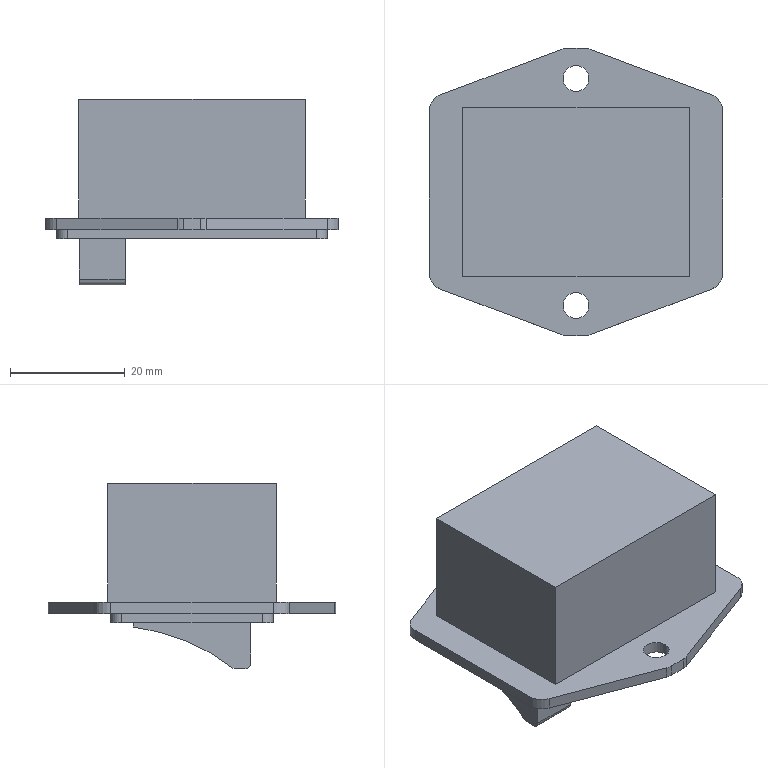Part | SolidWorks | features MirrorStock 1 | 1 solid | 50 faces | box 51 x 50 x 32.3 mm | volume 28039 mm3 | plane 32 | cylinder 18 | commonest cylinder face diameters 6 x8 4 x4 4.5 x4 2 x1 73.633 x1
STEP:
#1=CARTESIAN_POINT('',(2.25,-19.75,-20.7));
#2=VERTEX_POINT('',#1);
#3=CARTESIAN_POINT('',(-2.25,-19.75,-20.7));
#4=VERTEX_POINT('',#3);
#5=CARTESIAN_POINT('',(0.,-19.75,-20.7));
#6=DIRECTION('',(0.,0.,1.));
#7=DIRECTION('',(1.,0.,0.));
#8=AXIS2_PLACEMENT_3D('',#5,#6,#7);
#9=CIRCLE('',#8,2.25);
#10=EDGE_CURVE('',#2,#4,#9,.T.);
#11=ORIENTED_EDGE('',*,*,#10,.T.);
#12=CARTESIAN_POINT('',(-2.25,-19.75,-22.7));
#13=VERTEX_POINT('',#12);
#14=CARTESIAN_POINT('',(-2.25,-19.75,0.));
#15=DIRECTION('',(0.,0.,-1.));
#16=VECTOR('',#15,1000.);
#17=LINE('',#14,#16);
#18=EDGE_CURVE('',#4,#13,#17,.T.);
#19=ORIENTED_EDGE('',*,*,#18,.T.);
#20=CARTESIAN_POINT('',(2.25,-19.75,-22.7));
#21=VERTEX_POINT('',#20);
#22=CARTESIAN_POINT('',(0.,-19.75,-22.7));
#23=DIRECTION('',(0.,0.,1.));
#24=DIRECTION('',(1.,0.,0.));
#25=AXIS2_PLACEMENT_3D('',#22,#23,#24);
#26=CIRCLE('',#25,2.25);
#27=EDGE_CURVE('',#21,#13,#26,.T.);
#28=ORIENTED_EDGE('',*,*,#27,.F.);
#29=CARTESIAN_POINT('',(2.25,-19.75,0.));
#30=DIRECTION('',(0.,0.,-1.));
#31=VECTOR('',#30,1000.);
#32=LINE('',#29,#31);
#33=EDGE_CURVE('',#2,#21,#32,.T.);
#34=ORIENTED_EDGE('',*,*,#33,.F.);
#35=EDGE_LOOP('',(#11,#19,#28,#34));
#36=FACE_OUTER_BOUND('',#35,.T.);
#37=CARTESIAN_POINT('',(0.,-19.75,0.));
#38=DIRECTION('',(0.,0.,-1.));
#39=DIRECTION('',(1.,0.,0.));
#40=AXIS2_PLACEMENT_3D('',#37,#38,#39);
#41=CYLINDRICAL_SURFACE('',#40,2.25);
#42=ADVANCED_FACE('',(#36),#41,.F.);
#43=CARTESIAN_POINT('',(2.25,19.75,-20.7));
#44=VERTEX_POINT('',#43);
#45=CARTESIAN_POINT('',(-2.25,19.75,-20.7));
#46=VERTEX_POINT('',#45);
#47=CARTESIAN_POINT('',(0.,19.75,-20.7));
#48=DIRECTION('',(0.,0.,1.));
#49=DIRECTION('',(1.,0.,0.));
#50=AXIS2_PLACEMENT_3D('',#47,#48,#49);
#51=CIRCLE('',#50,2.25);
#52=EDGE_CURVE('',#44,#46,#51,.T.);
#53=ORIENTED_EDGE('',*,*,#52,.T.);
#54=CARTESIAN_POINT('',(-2.25,19.75,-22.7));
#55=VERTEX_POINT('',#54);
#56=CARTESIAN_POINT('',(-2.25,19.75,0.));
#57=DIRECTION('',(0.,0.,-1.));
#58=VECTOR('',#57,1000.);
#59=LINE('',#56,#58);
#60=EDGE_CURVE('',#46,#55,#59,.T.);
#61=ORIENTED_EDGE('',*,*,#60,.T.);
#62=CARTESIAN_POINT('',(2.25,19.75,-22.7));
#63=VERTEX_POINT('',#62);
#64=CARTESIAN_POINT('',(0.,19.75,-22.7));
#65=DIRECTION('',(0.,0.,1.));
#66=DIRECTION('',(1.,0.,0.));
#67=AXIS2_PLACEMENT_3D('',#64,#65,#66);
#68=CIRCLE('',#67,2.25);
#69=EDGE_CURVE('',#63,#55,#68,.T.);
#70=ORIENTED_EDGE('',*,*,#69,.F.);
#71=CARTESIAN_POINT('',(2.25,19.75,0.));
#72=DIRECTION('',(0.,0.,-1.));
#73=VECTOR('',#72,1000.);
#74=LINE('',#71,#73);
#75=EDGE_CURVE('',#44,#63,#74,.T.);
#76=ORIENTED_EDGE('',*,*,#75,.F.);
#77=EDGE_LOOP('',(#53,#61,#70,#76));
#78=FACE_OUTER_BOUND('',#77,.T.);
#79=CARTESIAN_POINT('',(0.,19.75,0.));
#80=DIRECTION('',(0.,0.,-1.));
#81=DIRECTION('',(1.,0.,0.));
#82=AXIS2_PLACEMENT_3D('',#79,#80,#81);
#83=CYLINDRICAL_SURFACE('',#82,2.25);
#84=ADVANCED_FACE('',(#78),#83,.F.);
#85=CARTESIAN_POINT('',(-21.6,-14.2,-24.3));
#86=VERTEX_POINT('',#85);
#87=CARTESIAN_POINT('',(21.6,-14.2,-24.3));
#88=VERTEX_POINT('',#87);
#89=CARTESIAN_POINT('',(23.6,-14.2,-24.3));
#90=DIRECTION('',(1.,0.,0.));
#91=VECTOR('',#90,1000.);
#92=LINE('',#89,#91);
#93=EDGE_CURVE('',#86,#88,#92,.T.);
#94=ORIENTED_EDGE('',*,*,#93,.F.);
#95=CARTESIAN_POINT('',(-23.6,-12.2,-24.3));
#96=VERTEX_POINT('',#95);
#97=CARTESIAN_POINT('',(-21.6,-12.2,-24.3));
#98=DIRECTION('',(0.,0.,1.));
#99=DIRECTION('',(1.,0.,0.));
#100=AXIS2_PLACEMENT_3D('',#97,#98,#99);
#101=CIRCLE('',#100,2.);
#102=EDGE_CURVE('',#96,#86,#101,.T.);
#103=ORIENTED_EDGE('',*,*,#102,.F.);
#104=CARTESIAN_POINT('',(-23.6,12.2,-24.3));
#105=VERTEX_POINT('',#104);
#106=CARTESIAN_POINT('',(-23.6,-14.2,-24.3));
#107=DIRECTION('',(0.,-1.,0.));
#108=VECTOR('',#107,1000.);
#109=LINE('',#106,#108);
#110=EDGE_CURVE('',#105,#96,#109,.T.);
#111=ORIENTED_EDGE('',*,*,#110,.F.);
#112=CARTESIAN_POINT('',(-21.6,14.2,-24.3));
#113=VERTEX_POINT('',#112);
#114=CARTESIAN_POINT('',(-21.6,12.2,-24.3));
#115=DIRECTION('',(0.,0.,1.));
#116=DIRECTION('',(1.,0.,0.));
#117=AXIS2_PLACEMENT_3D('',#114,#115,#116);
#118=CIRCLE('',#117,2.);
#119=EDGE_CURVE('',#113,#105,#118,.T.);
#120=ORIENTED_EDGE('',*,*,#119,.F.);
#121=CARTESIAN_POINT('',(21.6,14.2,-24.3));
#122=VERTEX_POINT('',#121);
#123=CARTESIAN_POINT('',(23.6,14.2,-24.3));
#124=DIRECTION('',(-1.,0.,0.));
#125=VECTOR('',#124,1000.);
#126=LINE('',#123,#125);
#127=EDGE_CURVE('',#122,#113,#126,.T.);
#128=ORIENTED_EDGE('',*,*,#127,.F.);
#129=CARTESIAN_POINT('',(23.6,12.2,-24.3));
#130=VERTEX_POINT('',#129);
#131=CARTESIAN_POINT('',(21.6,12.2,-24.3));
#132=DIRECTION('',(0.,0.,1.));
#133=DIRECTION('',(1.,0.,0.));
#134=AXIS2_PLACEMENT_3D('',#131,#132,#133);
#135=CIRCLE('',#134,2.);
#136=EDGE_CURVE('',#130,#122,#135,.T.);
#137=ORIENTED_EDGE('',*,*,#136,.F.);
#138=CARTESIAN_POINT('',(23.6,-12.2,-24.3));
#139=VERTEX_POINT('',#138);
#140=CARTESIAN_POINT('',(23.6,-14.2,-24.3));
#141=DIRECTION('',(0.,1.,0.));
#142=VECTOR('',#141,1000.);
#143=LINE('',#140,#142);
#144=EDGE_CURVE('',#139,#130,#143,.T.);
#145=ORIENTED_EDGE('',*,*,#144,.F.);
#146=CARTESIAN_POINT('',(21.6,-12.2,-24.3));
#147=DIRECTION('',(0.,0.,1.));
#148=DIRECTION('',(1.,0.,0.));
#149=AXIS2_PLACEMENT_3D('',#146,#147,#148);
#150=CIRCLE('',#149,2.);
#151=EDGE_CURVE('',#88,#139,#150,.T.);
#152=ORIENTED_EDGE('',*,*,#151,.F.);
#153=EDGE_LOOP('',(#94,#103,#111,#120,#128,#137,#145,#152));
#154=FACE_OUTER_BOUND('',#153,.T.);
#155=CARTESIAN_POINT('',(2.9,12.2,-24.3));
#156=VERTEX_POINT('',#155);
#157=CARTESIAN_POINT('',(2.9,-12.2,-24.3));
#158=VERTEX_POINT('',#157);
#159=CARTESIAN_POINT('',(2.9,0.,-24.3));
#160=DIRECTION('',(0.,-1.,0.));
#161=VECTOR('',#160,1000.);
#162=LINE('',#159,#161);
#163=EDGE_CURVE('',#156,#158,#162,.T.);
#164=ORIENTED_EDGE('',*,*,#163,.T.);
#165=CARTESIAN_POINT('',(15.9,-12.2,-24.3));
#166=VERTEX_POINT('',#165);
#167=CARTESIAN_POINT('',(0.,-12.2,-24.3));
#168=DIRECTION('',(1.,0.,0.));
#169=VECTOR('',#168,1000.);
#170=LINE('',#167,#169);
#171=EDGE_CURVE('',#158,#166,#170,.T.);
#172=ORIENTED_EDGE('',*,*,#171,.T.);
#173=CARTESIAN_POINT('',(18.9,-7.5,-24.3));
#174=VERTEX_POINT('',#173);
#175=CARTESIAN_POINT('',(16.83,-10.743,-24.3));
#176=DIRECTION('',(0.538,0.8429,0.));
#177=VECTOR('',#176,1000.);
#178=LINE('',#175,#177);
#179=EDGE_CURVE('',#166,#174,#178,.T.);
#180=ORIENTED_EDGE('',*,*,#179,.T.);
#181=CARTESIAN_POINT('',(18.9,7.5,-24.3));
#182=VERTEX_POINT('',#181);
#183=CARTESIAN_POINT('',(18.9,0.,-24.3));
#184=DIRECTION('',(0.,1.,0.));
#185=VECTOR('',#184,1000.);
#186=LINE('',#183,#185);
#187=EDGE_CURVE('',#174,#182,#186,.T.);
#188=ORIENTED_EDGE('',*,*,#187,.T.);
#189=CARTESIAN_POINT('',(15.9,12.2,-24.3));
#190=VERTEX_POINT('',#189);
#191=CARTESIAN_POINT('',(16.83,10.743,-24.3));
#192=DIRECTION('',(-0.538,0.8429,0.));
#193=VECTOR('',#192,1000.);
#194=LINE('',#191,#193);
#195=EDGE_CURVE('',#182,#190,#194,.T.);
#196=ORIENTED_EDGE('',*,*,#195,.T.);
#197=CARTESIAN_POINT('',(0.,12.2,-24.3));
#198=DIRECTION('',(1.,0.,0.));
#199=VECTOR('',#198,1000.);
#200=LINE('',#197,#199);
#201=EDGE_CURVE('',#156,#190,#200,.T.);
#202=ORIENTED_EDGE('',*,*,#201,.F.);
#203=EDGE_LOOP('',(#164,#172,#180,#188,#196,#202));
#204=FACE_BOUND('',#203,.T.);
#205=CARTESIAN_POINT('',(-19.6,-10.2,-24.3));
#206=VERTEX_POINT('',#205);
#207=CARTESIAN_POINT('',(-11.6,-10.2,-24.3));
#208=VERTEX_POINT('',#207);
#209=CARTESIAN_POINT('',(-19.6,-10.2,-24.3));
#210=DIRECTION('',(1.,0.,0.));
#211=VECTOR('',#210,1000.);
#212=LINE('',#209,#211);
#213=EDGE_CURVE('',#206,#208,#212,.T.);
#214=ORIENTED_EDGE('',*,*,#213,.T.);
#215=CARTESIAN_POINT('',(-11.6,10.2,-24.3));
#216=VERTEX_POINT('',#215);
#217=CARTESIAN_POINT('',(-11.6,10.2,-24.3));
#218=DIRECTION('',(0.,1.,0.));
#219=VECTOR('',#218,1000.);
#220=LINE('',#217,#219);
#221=EDGE_CURVE('',#208,#216,#220,.T.);
#222=ORIENTED_EDGE('',*,*,#221,.T.);
#223=CARTESIAN_POINT('',(-19.6,10.2,-24.3));
#224=VERTEX_POINT('',#223);
#225=CARTESIAN_POINT('',(-19.6,10.2,-24.3));
#226=DIRECTION('',(-1.,0.,0.));
#227=VECTOR('',#226,1000.);
#228=LINE('',#225,#227);
#229=EDGE_CURVE('',#216,#224,#228,.T.);
#230=ORIENTED_EDGE('',*,*,#229,.T.);
#231=CARTESIAN_POINT('',(-19.6,10.2,-24.3));
#232=DIRECTION('',(0.,-1.,0.));
#233=VECTOR('',#232,1000.);
#234=LINE('',#231,#233);
#235=EDGE_CURVE('',#224,#206,#234,.T.);
#236=ORIENTED_EDGE('',*,*,#235,.T.);
#237=EDGE_LOOP('',(#214,#222,#230,#236));
#238=FACE_BOUND('',#237,.T.);
#239=CARTESIAN_POINT('',(0.,0.,-24.3));
#240=DIRECTION('',(0.,0.,-1.));
#241=DIRECTION('',(1.,0.,0.));
#242=AXIS2_PLACEMENT_3D('',#239,#240,#241);
#243=PLANE('',#242);
#244=ADVANCED_FACE('',(#154,#204,#238),#243,.T.);
#245=CARTESIAN_POINT('',(-23.552,-16.929,-22.7));
#246=VERTEX_POINT('',#245);
#247=CARTESIAN_POINT('',(-2.509,-24.809,-22.7));
#248=VERTEX_POINT('',#247);
#249=CARTESIAN_POINT('',(-8.456,-22.582,-22.7));
#250=DIRECTION('',(0.9365,-0.3507,0.));
#251=VECTOR('',#250,1000.);
#252=LINE('',#249,#251);
#253=EDGE_CURVE('',#246,#248,#252,.T.);
#254=ORIENTED_EDGE('',*,*,#253,.F.);
#255=CARTESIAN_POINT('',(-25.5,-14.12,-22.7));
#256=VERTEX_POINT('',#255);
#257=CARTESIAN_POINT('',(-22.5,-14.12,-22.7));
#258=DIRECTION('',(0.,0.,1.));
#259=DIRECTION('',(1.,0.,0.));
#260=AXIS2_PLACEMENT_3D('',#257,#258,#259);
#261=CIRCLE('',#260,3.);
#262=EDGE_CURVE('',#256,#246,#261,.T.);
#263=ORIENTED_EDGE('',*,*,#262,.F.);
#264=CARTESIAN_POINT('',(-25.5,14.12,-22.7));
#265=VERTEX_POINT('',#264);
#266=CARTESIAN_POINT('',(-25.5,-25.,-22.7));
#267=DIRECTION('',(0.,-1.,0.));
#268=VECTOR('',#267,1000.);
#269=LINE('',#266,#268);
#270=EDGE_CURVE('',#265,#256,#269,.T.);
#271=ORIENTED_EDGE('',*,*,#270,.F.);
#272=CARTESIAN_POINT('',(-23.552,16.929,-22.7));
#273=VERTEX_POINT('',#272);
#274=CARTESIAN_POINT('',(-22.5,14.12,-22.7));
#275=DIRECTION('',(0.,0.,1.));
#276=DIRECTION('',(1.,0.,0.));
#277=AXIS2_PLACEMENT_3D('',#274,#275,#276);
#278=CIRCLE('',#277,3.);
#279=EDGE_CURVE('',#273,#265,#278,.T.);
#280=ORIENTED_EDGE('',*,*,#279,.F.);
#281=CARTESIAN_POINT('',(-2.509,24.809,-22.7));
#282=VERTEX_POINT('',#281);
#283=CARTESIAN_POINT('',(-8.456,22.582,-22.7));
#284=DIRECTION('',(0.9365,0.3507,0.));
#285=VECTOR('',#284,1000.);
#286=LINE('',#283,#285);
#287=EDGE_CURVE('',#273,#282,#286,.T.);
#288=ORIENTED_EDGE('',*,*,#287,.T.);
#289=CARTESIAN_POINT('',(-1.457,25.,-22.7));
#290=VERTEX_POINT('',#289);
#291=CARTESIAN_POINT('',(-1.457,22.,-22.7));
#292=DIRECTION('',(0.,0.,1.));
#293=DIRECTION('',(1.,0.,0.));
#294=AXIS2_PLACEMENT_3D('',#291,#292,#293);
#295=CIRCLE('',#294,3.);
#296=EDGE_CURVE('',#290,#282,#295,.T.);
#297=ORIENTED_EDGE('',*,*,#296,.F.);
#298=CARTESIAN_POINT('',(1.457,25.,-22.7));
#299=VERTEX_POINT('',#298);
#300=CARTESIAN_POINT('',(25.5,25.,-22.7));
#301=DIRECTION('',(-1.,0.,0.));
#302=VECTOR('',#301,1000.);
#303=LINE('',#300,#302);
#304=EDGE_CURVE('',#299,#290,#303,.T.);
#305=ORIENTED_EDGE('',*,*,#304,.F.);
#306=CARTESIAN_POINT('',(2.509,24.809,-22.7));
#307=VERTEX_POINT('',#306);
#308=CARTESIAN_POINT('',(1.457,22.,-22.7));
#309=DIRECTION('',(0.,0.,1.));
#310=DIRECTION('',(1.,0.,0.));
#311=AXIS2_PLACEMENT_3D('',#308,#309,#310);
#312=CIRCLE('',#311,3.);
#313=EDGE_CURVE('',#307,#299,#312,.T.);
#314=ORIENTED_EDGE('',*,*,#313,.F.);
#315=CARTESIAN_POINT('',(23.552,16.929,-22.7));
#316=VERTEX_POINT('',#315);
#317=CARTESIAN_POINT('',(8.456,22.582,-22.7));
#318=DIRECTION('',(-0.9365,0.3507,0.));
#319=VECTOR('',#318,1000.);
#320=LINE('',#317,#319);
#321=EDGE_CURVE('',#316,#307,#320,.T.);
#322=ORIENTED_EDGE('',*,*,#321,.F.);
#323=CARTESIAN_POINT('',(25.5,14.12,-22.7));
#324=VERTEX_POINT('',#323);
#325=CARTESIAN_POINT('',(22.5,14.12,-22.7));
#326=DIRECTION('',(0.,0.,1.));
#327=DIRECTION('',(1.,0.,0.));
#328=AXIS2_PLACEMENT_3D('',#325,#326,#327);
#329=CIRCLE('',#328,3.);
#330=EDGE_CURVE('',#324,#316,#329,.T.);
#331=ORIENTED_EDGE('',*,*,#330,.F.);
#332=CARTESIAN_POINT('',(25.5,-14.12,-22.7));
#333=VERTEX_POINT('',#332);
#334=CARTESIAN_POINT('',(25.5,-25.,-22.7));
#335=DIRECTION('',(0.,1.,0.));
#336=VECTOR('',#335,1000.);
#337=LINE('',#334,#336);
#338=EDGE_CURVE('',#333,#324,#337,.T.);
#339=ORIENTED_EDGE('',*,*,#338,.F.);
#340=CARTESIAN_POINT('',(23.552,-16.929,-22.7));
#341=VERTEX_POINT('',#340);
#342=CARTESIAN_POINT('',(22.5,-14.12,-22.7));
#343=DIRECTION('',(0.,0.,1.));
#344=DIRECTION('',(1.,0.,0.));
#345=AXIS2_PLACEMENT_3D('',#342,#343,#344);
#346=CIRCLE('',#345,3.);
#347=EDGE_CURVE('',#341,#333,#346,.T.);
#348=ORIENTED_EDGE('',*,*,#347,.F.);
#349=CARTESIAN_POINT('',(2.509,-24.809,-22.7));
#350=VERTEX_POINT('',#349);
#351=CARTESIAN_POINT('',(8.456,-22.582,-22.7));
#352=DIRECTION('',(-0.9365,-0.3507,0.));
#353=VECTOR('',#352,1000.);
#354=LINE('',#351,#353);
#355=EDGE_CURVE('',#341,#350,#354,.T.);
#356=ORIENTED_EDGE('',*,*,#355,.T.);
#357=CARTESIAN_POINT('',(1.457,-25.,-22.7));
#358=VERTEX_POINT('',#357);
#359=CARTESIAN_POINT('',(1.457,-22.,-22.7));
#360=DIRECTION('',(0.,0.,1.));
#361=DIRECTION('',(1.,0.,0.));
#362=AXIS2_PLACEMENT_3D('',#359,#360,#361);
#363=CIRCLE('',#362,3.);
#364=EDGE_CURVE('',#358,#350,#363,.T.);
#365=ORIENTED_EDGE('',*,*,#364,.F.);
#366=CARTESIAN_POINT('',(-1.457,-25.,-22.7));
#367=VERTEX_POINT('',#366);
#368=CARTESIAN_POINT('',(25.5,-25.,-22.7));
#369=DIRECTION('',(1.,0.,0.));
#370=VECTOR('',#369,1000.);
#371=LINE('',#368,#370);
#372=EDGE_CURVE('',#367,#358,#371,.T.);
#373=ORIENTED_EDGE('',*,*,#372,.F.);
#374=CARTESIAN_POINT('',(-1.457,-22.,-22.7));
#375=DIRECTION('',(0.,0.,1.));
#376=DIRECTION('',(1.,0.,0.));
#377=AXIS2_PLACEMENT_3D('',#374,#375,#376);
#378=CIRCLE('',#377,3.);
#379=EDGE_CURVE('',#248,#367,#378,.T.);
#380=ORIENTED_EDGE('',*,*,#379,.F.);
#381=EDGE_LOOP('',(#254,#263,#271,#280,#288,#297,#305,#314,#322,#331,#339,#348,#356,#365,#373,#380));
#382=FACE_OUTER_BOUND('',#381,.T.);
#383=ORIENTED_EDGE('',*,*,#27,.T.);
#384=CARTESIAN_POINT('',(0.,-19.75,-22.7));
#385=DIRECTION('',(0.,0.,1.));
#386=DIRECTION('',(1.,0.,0.));
#387=AXIS2_PLACEMENT_3D('',#384,#385,#386);
#388=CIRCLE('',#387,2.25);
#389=EDGE_CURVE('',#13,#21,#388,.T.);
#390=ORIENTED_EDGE('',*,*,#389,.T.);
#391=EDGE_LOOP('',(#383,#390));
#392=FACE_BOUND('',#391,.T.);
#393=ORIENTED_EDGE('',*,*,#69,.T.);
#394=CARTESIAN_POINT('',(0.,19.75,-22.7));
#395=DIRECTION('',(0.,0.,1.));
#396=DIRECTION('',(1.,0.,0.));
#397=AXIS2_PLACEMENT_3D('',#394,#395,#396);
#398=CIRCLE('',#397,2.25);
#399=EDGE_CURVE('',#55,#63,#398,.T.);
#400=ORIENTED_EDGE('',*,*,#399,.T.);
#401=EDGE_LOOP('',(#393,#400));
#402=FACE_BOUND('',#401,.T.);
#403=CARTESIAN_POINT('',(-21.6,-14.2,-22.7));
#404=VERTEX_POINT('',#403);
#405=CARTESIAN_POINT('',(21.6,-14.2,-22.7));
#406=VERTEX_POINT('',#405);
#407=CARTESIAN_POINT('',(23.6,-14.2,-22.7));
#408=DIRECTION('',(1.,0.,0.));
#409=VECTOR('',#408,1000.);
#410=LINE('',#407,#409);
#411=EDGE_CURVE('',#404,#406,#410,.T.);
#412=ORIENTED_EDGE('',*,*,#411,.T.);
#413=CARTESIAN_POINT('',(23.6,-12.2,-22.7));
#414=VERTEX_POINT('',#413);
#415=CARTESIAN_POINT('',(21.6,-12.2,-22.7));
#416=DIRECTION('',(0.,0.,-1.));
#417=DIRECTION('',(1.,0.,0.));
#418=AXIS2_PLACEMENT_3D('',#415,#416,#417);
#419=CIRCLE('',#418,2.);
#420=EDGE_CURVE('',#414,#406,#419,.T.);
#421=ORIENTED_EDGE('',*,*,#420,.F.);
#422=CARTESIAN_POINT('',(23.6,12.2,-22.7));
#423=VERTEX_POINT('',#422);
#424=CARTESIAN_POINT('',(23.6,-14.2,-22.7));
#425=DIRECTION('',(0.,1.,0.));
#426=VECTOR('',#425,1000.);
#427=LINE('',#424,#426);
#428=EDGE_CURVE('',#414,#423,#427,.T.);
#429=ORIENTED_EDGE('',*,*,#428,.T.);
#430=CARTESIAN_POINT('',(21.6,14.2,-22.7));
#431=VERTEX_POINT('',#430);
#432=CARTESIAN_POINT('',(21.6,12.2,-22.7));
#433=DIRECTION('',(0.,0.,-1.));
#434=DIRECTION('',(1.,0.,0.));
#435=AXIS2_PLACEMENT_3D('',#432,#433,#434);
#436=CIRCLE('',#435,2.);
#437=EDGE_CURVE('',#431,#423,#436,.T.);
#438=ORIENTED_EDGE('',*,*,#437,.F.);
#439=CARTESIAN_POINT('',(-21.6,14.2,-22.7));
#440=VERTEX_POINT('',#439);
#441=CARTESIAN_POINT('',(23.6,14.2,-22.7));
#442=DIRECTION('',(-1.,0.,0.));
#443=VECTOR('',#442,1000.);
#444=LINE('',#441,#443);
#445=EDGE_CURVE('',#431,#440,#444,.T.);
#446=ORIENTED_EDGE('',*,*,#445,.T.);
#447=CARTESIAN_POINT('',(-23.6,12.2,-22.7));
#448=VERTEX_POINT('',#447);
#449=CARTESIAN_POINT('',(-21.6,12.2,-22.7));
#450=DIRECTION('',(0.,0.,-1.));
#451=DIRECTION('',(1.,0.,0.));
#452=AXIS2_PLACEMENT_3D('',#449,#450,#451);
#453=CIRCLE('',#452,2.);
#454=EDGE_CURVE('',#448,#440,#453,.T.);
#455=ORIENTED_EDGE('',*,*,#454,.F.);
#456=CARTESIAN_POINT('',(-23.6,-12.2,-22.7));
#457=VERTEX_POINT('',#456);
#458=CARTESIAN_POINT('',(-23.6,-14.2,-22.7));
#459=DIRECTION('',(0.,-1.,0.));
#460=VECTOR('',#459,1000.);
#461=LINE('',#458,#460);
#462=EDGE_CURVE('',#448,#457,#461,.T.);
#463=ORIENTED_EDGE('',*,*,#462,.T.);
#464=CARTESIAN_POINT('',(-21.6,-12.2,-22.7));
#465=DIRECTION('',(0.,0.,-1.));
#466=DIRECTION('',(1.,0.,0.));
#467=AXIS2_PLACEMENT_3D('',#464,#465,#466);
#468=CIRCLE('',#467,2.);
#469=EDGE_CURVE('',#404,#457,#468,.T.);
#470=ORIENTED_EDGE('',*,*,#469,.F.);
#471=EDGE_LOOP('',(#412,#421,#429,#438,#446,#455,#463,#470));
#472=FACE_BOUND('',#471,.T.);
#473=CARTESIAN_POINT('',(0.,0.,-22.7));
#474=DIRECTION('',(0.,0.,-1.));
#475=DIRECTION('',(1.,0.,0.));
#476=AXIS2_PLACEMENT_3D('',#473,#474,#475);
#477=PLANE('',#476);
#478=ADVANCED_FACE('',(#382,#392,#402,#472),#477,.T.);
#479=ORIENTED_EDGE('',*,*,#10,.F.);
#480=CARTESIAN_POINT('',(0.,-19.75,-20.7));
#481=DIRECTION('',(0.,0.,1.));
#482=DIRECTION('',(1.,0.,0.));
#483=AXIS2_PLACEMENT_3D('',#480,#481,#482);
#484=CIRCLE('',#483,2.25);
#485=EDGE_CURVE('',#4,#2,#484,.T.);
#486=ORIENTED_EDGE('',*,*,#485,.F.);
#487=EDGE_LOOP('',(#479,#486));
#488=FACE_BOUND('',#487,.T.);
#489=ORIENTED_EDGE('',*,*,#52,.F.);
#490=CARTESIAN_POINT('',(0.,19.75,-20.7));
#491=DIRECTION('',(0.,0.,1.));
#492=DIRECTION('',(1.,0.,0.));
#493=AXIS2_PLACEMENT_3D('',#490,#491,#492);
#494=CIRCLE('',#493,2.25);
#495=EDGE_CURVE('',#46,#44,#494,.T.);
#496=ORIENTED_EDGE('',*,*,#495,.F.);
#497=EDGE_LOOP('',(#489,#496));
#498=FACE_BOUND('',#497,.T.);
#499=CARTESIAN_POINT('',(19.75,14.7,-20.7));
#500=VERTEX_POINT('',#499);
#501=CARTESIAN_POINT('',(-19.75,14.7,-20.7));
#502=VERTEX_POINT('',#501);
#503=CARTESIAN_POINT('',(19.75,14.7,-20.7));
#504=DIRECTION('',(-1.,0.,0.));
#505=VECTOR('',#504,1000.);
#506=LINE('',#503,#505);
#507=EDGE_CURVE('',#500,#502,#506,.T.);
#508=ORIENTED_EDGE('',*,*,#507,.F.);
#509=CARTESIAN_POINT('',(19.75,-14.7,-20.7));
#510=VERTEX_POINT('',#509);
#511=CARTESIAN_POINT('',(19.75,-14.7,-20.7));
#512=DIRECTION('',(0.,1.,0.));
#513=VECTOR('',#512,1000.);
#514=LINE('',#511,#513);
#515=EDGE_CURVE('',#510,#500,#514,.T.);
#516=ORIENTED_EDGE('',*,*,#515,.F.);
#517=CARTESIAN_POINT('',(-19.75,-14.7,-20.7));
#518=VERTEX_POINT('',#517);
#519=CARTESIAN_POINT('',(19.75,-14.7,-20.7));
#520=DIRECTION('',(1.,0.,0.));
#521=VECTOR('',#520,1000.);
#522=LINE('',#519,#521);
#523=EDGE_CURVE('',#518,#510,#522,.T.);
#524=ORIENTED_EDGE('',*,*,#523,.F.);
#525=CARTESIAN_POINT('',(-19.75,-14.7,-20.7));
#526=DIRECTION('',(0.,-1.,0.));
#527=VECTOR('',#526,1000.);
#528=LINE('',#525,#527);
#529=EDGE_CURVE('',#502,#518,#528,.T.);
#530=ORIENTED_EDGE('',*,*,#529,.F.);
#531=EDGE_LOOP('',(#508,#516,#524,#530));
#532=FACE_BOUND('',#531,.T.);
#533=CARTESIAN_POINT('',(-1.457,-25.,-20.7));
#534=VERTEX_POINT('',#533);
#535=CARTESIAN_POINT('',(1.457,-25.,-20.7));
#536=VERTEX_POINT('',#535);
#537=CARTESIAN_POINT('',(25.5,-25.,-20.7));
#538=DIRECTION('',(1.,0.,0.));
#539=VECTOR('',#538,1000.);
#540=LINE('',#537,#539);
#541=EDGE_CURVE('',#534,#536,#540,.T.);
#542=ORIENTED_EDGE('',*,*,#541,.T.);
#543=CARTESIAN_POINT('',(2.509,-24.809,-20.7));
#544=VERTEX_POINT('',#543);
#545=CARTESIAN_POINT('',(1.457,-22.,-20.7));
#546=DIRECTION('',(0.,0.,-1.));
#547=DIRECTION('',(1.,0.,0.));
#548=AXIS2_PLACEMENT_3D('',#545,#546,#547);
#549=CIRCLE('',#548,3.);
#550=EDGE_CURVE('',#544,#536,#549,.T.);
#551=ORIENTED_EDGE('',*,*,#550,.F.);
#552=CARTESIAN_POINT('',(23.552,-16.929,-20.7));
#553=VERTEX_POINT('',#552);
#554=CARTESIAN_POINT('',(8.456,-22.582,-20.7));
#555=DIRECTION('',(-0.9365,-0.3507,0.));
#556=VECTOR('',#555,1000.);
#557=LINE('',#554,#556);
#558=EDGE_CURVE('',#553,#544,#557,.T.);
#559=ORIENTED_EDGE('',*,*,#558,.F.);
#560=CARTESIAN_POINT('',(25.5,-14.12,-20.7));
#561=VERTEX_POINT('',#560);
#562=CARTESIAN_POINT('',(22.5,-14.12,-20.7));
#563=DIRECTION('',(0.,0.,-1.));
#564=DIRECTION('',(1.,0.,0.));
#565=AXIS2_PLACEMENT_3D('',#562,#563,#564);
#566=CIRCLE('',#565,3.);
#567=EDGE_CURVE('',#561,#553,#566,.T.);
#568=ORIENTED_EDGE('',*,*,#567,.F.);
#569=CARTESIAN_POINT('',(25.5,14.12,-20.7));
#570=VERTEX_POINT('',#569);
#571=CARTESIAN_POINT('',(25.5,-25.,-20.7));
#572=DIRECTION('',(0.,1.,0.));
#573=VECTOR('',#572,1000.);
#574=LINE('',#571,#573);
#575=EDGE_CURVE('',#561,#570,#574,.T.);
#576=ORIENTED_EDGE('',*,*,#575,.T.);
#577=CARTESIAN_POINT('',(23.552,16.929,-20.7));
#578=VERTEX_POINT('',#577);
#579=CARTESIAN_POINT('',(22.5,14.12,-20.7));
#580=DIRECTION('',(0.,0.,-1.));
#581=DIRECTION('',(1.,0.,0.));
#582=AXIS2_PLACEMENT_3D('',#579,#580,#581);
#583=CIRCLE('',#582,3.);
#584=EDGE_CURVE('',#578,#570,#583,.T.);
#585=ORIENTED_EDGE('',*,*,#584,.F.);
#586=CARTESIAN_POINT('',(2.509,24.809,-20.7));
#587=VERTEX_POINT('',#586);
#588=CARTESIAN_POINT('',(8.456,22.582,-20.7));
#589=DIRECTION('',(-0.9365,0.3507,0.));
#590=VECTOR('',#589,1000.);
#591=LINE('',#588,#590);
#592=EDGE_CURVE('',#578,#587,#591,.T.);
#593=ORIENTED_EDGE('',*,*,#592,.T.);
#594=CARTESIAN_POINT('',(1.457,25.,-20.7));
#595=VERTEX_POINT('',#594);
#596=CARTESIAN_POINT('',(1.457,22.,-20.7));
#597=DIRECTION('',(0.,0.,-1.));
#598=DIRECTION('',(1.,0.,0.));
#599=AXIS2_PLACEMENT_3D('',#596,#597,#598);
#600=CIRCLE('',#599,3.);
#601=EDGE_CURVE('',#595,#587,#600,.T.);
#602=ORIENTED_EDGE('',*,*,#601,.F.);
#603=CARTESIAN_POINT('',(-1.457,25.,-20.7));
#604=VERTEX_POINT('',#603);
#605=CARTESIAN_POINT('',(25.5,25.,-20.7));
#606=DIRECTION('',(-1.,0.,0.));
#607=VECTOR('',#606,1000.);
#608=LINE('',#605,#607);
#609=EDGE_CURVE('',#595,#604,#608,.T.);
#610=ORIENTED_EDGE('',*,*,#609,.T.);
#611=CARTESIAN_POINT('',(-2.509,24.809,-20.7));
#612=VERTEX_POINT('',#611);
#613=CARTESIAN_POINT('',(-1.457,22.,-20.7));
#614=DIRECTION('',(0.,0.,-1.));
#615=DIRECTION('',(1.,0.,0.));
#616=AXIS2_PLACEMENT_3D('',#613,#614,#615);
#617=CIRCLE('',#616,3.);
#618=EDGE_CURVE('',#612,#604,#617,.T.);
#619=ORIENTED_EDGE('',*,*,#618,.F.);
#620=CARTESIAN_POINT('',(-23.552,16.929,-20.7));
#621=VERTEX_POINT('',#620);
#622=CARTESIAN_POINT('',(-8.456,22.582,-20.7));
#623=DIRECTION('',(0.9365,0.3507,0.));
#624=VECTOR('',#623,1000.);
#625=LINE('',#622,#624);
#626=EDGE_CURVE('',#621,#612,#625,.T.);
#627=ORIENTED_EDGE('',*,*,#626,.F.);
#628=CARTESIAN_POINT('',(-25.5,14.12,-20.7));
#629=VERTEX_POINT('',#628);
#630=CARTESIAN_POINT('',(-22.5,14.12,-20.7));
#631=DIRECTION('',(0.,0.,-1.));
#632=DIRECTION('',(1.,0.,0.));
#633=AXIS2_PLACEMENT_3D('',#630,#631,#632);
#634=CIRCLE('',#633,3.);
#635=EDGE_CURVE('',#629,#621,#634,.T.);
#636=ORIENTED_EDGE('',*,*,#635,.F.);
#637=CARTESIAN_POINT('',(-25.5,-14.12,-20.7));
#638=VERTEX_POINT('',#637);
#639=CARTESIAN_POINT('',(-25.5,-25.,-20.7));
#640=DIRECTION('',(0.,-1.,0.));
#641=VECTOR('',#640,1000.);
#642=LINE('',#639,#641);
#643=EDGE_CURVE('',#629,#638,#642,.T.);
#644=ORIENTED_EDGE('',*,*,#643,.T.);
#645=CARTESIAN_POINT('',(-23.552,-16.929,-20.7));
#646=VERTEX_POINT('',#645);
#647=CARTESIAN_POINT('',(-22.5,-14.12,-20.7));
#648=DIRECTION('',(0.,0.,-1.));
#649=DIRECTION('',(1.,0.,0.));
#650=AXIS2_PLACEMENT_3D('',#647,#648,#649);
#651=CIRCLE('',#650,3.);
#652=EDGE_CURVE('',#646,#638,#651,.T.);
#653=ORIENTED_EDGE('',*,*,#652,.F.);
#654=CARTESIAN_POINT('',(-2.509,-24.809,-20.7));
#655=VERTEX_POINT('',#654);
#656=CARTESIAN_POINT('',(-8.456,-22.582,-20.7));
#657=DIRECTION('',(0.9365,-0.3507,0.));
#658=VECTOR('',#657,1000.);
#659=LINE('',#656,#658);
#660=EDGE_CURVE('',#646,#655,#659,.T.);
#661=ORIENTED_EDGE('',*,*,#660,.T.);
#662=CARTESIAN_POINT('',(-1.457,-22.,-20.7));
#663=DIRECTION('',(0.,0.,-1.));
#664=DIRECTION('',(1.,0.,0.));
#665=AXIS2_PLACEMENT_3D('',#662,#663,#664);
#666=CIRCLE('',#665,3.);
#667=EDGE_CURVE('',#534,#655,#666,.T.);
#668=ORIENTED_EDGE('',*,*,#667,.F.);
#669=EDGE_LOOP('',(#542,#551,#559,#568,#576,#585,#593,#602,#610,#619,#627,#636,#644,#653,#661,#668));
#670=FACE_OUTER_BOUND('',#669,.T.);
#671=CARTESIAN_POINT('',(0.,0.,-20.7));
#672=DIRECTION('',(0.,0.,-1.));
#673=DIRECTION('',(1.,0.,0.));
#674=AXIS2_PLACEMENT_3D('',#671,#672,#673);
#675=PLANE('',#674);
#676=ADVANCED_FACE('',(#488,#498,#532,#670),#675,.F.);
#677=ORIENTED_EDGE('',*,*,#270,.T.);
#678=CARTESIAN_POINT('',(-25.5,-14.12,-22.7));
#679=DIRECTION('',(0.,0.,-1.));
#680=VECTOR('',#679,1000.);
#681=LINE('',#678,#680);
#682=EDGE_CURVE('',#638,#256,#681,.T.);
#683=ORIENTED_EDGE('',*,*,#682,.F.);
#684=ORIENTED_EDGE('',*,*,#643,.F.);
#685=CARTESIAN_POINT('',(-25.5,14.12,-22.7));
#686=DIRECTION('',(0.,0.,1.));
#687=VECTOR('',#686,1000.);
#688=LINE('',#685,#687);
#689=EDGE_CURVE('',#265,#629,#688,.T.);
#690=ORIENTED_EDGE('',*,*,#689,.F.);
#691=EDGE_LOOP('',(#677,#683,#684,#690));
#692=FACE_OUTER_BOUND('',#691,.T.);
#693=CARTESIAN_POINT('',(-25.5,-25.,-22.7));
#694=DIRECTION('',(1.,0.,0.));
#695=DIRECTION('',(0.,1.,0.));
#696=AXIS2_PLACEMENT_3D('',#693,#694,#695);
#697=PLANE('',#696);
#698=ADVANCED_FACE('',(#692),#697,.F.);
#699=ORIENTED_EDGE('',*,*,#372,.T.);
#700=CARTESIAN_POINT('',(1.457,-25.,-22.7));
#701=DIRECTION('',(0.,0.,-1.));
#702=VECTOR('',#701,1000.);
#703=LINE('',#700,#702);
#704=EDGE_CURVE('',#536,#358,#703,.T.);
#705=ORIENTED_EDGE('',*,*,#704,.F.);
#706=ORIENTED_EDGE('',*,*,#541,.F.);
#707=CARTESIAN_POINT('',(-1.457,-25.,-20.7));
#708=DIRECTION('',(0.,0.,1.));
#709=VECTOR('',#708,1000.);
#710=LINE('',#707,#709);
#711=EDGE_CURVE('',#367,#534,#710,.T.);
#712=ORIENTED_EDGE('',*,*,#711,.F.);
#713=EDGE_LOOP('',(#699,#705,#706,#712));
#714=FACE_OUTER_BOUND('',#713,.T.);
#715=CARTESIAN_POINT('',(25.5,-25.,-22.7));
#716=DIRECTION('',(0.,1.,0.));
#717=DIRECTION('',(-1.,0.,0.));
#718=AXIS2_PLACEMENT_3D('',#715,#716,#717);
#719=PLANE('',#718);
#720=ADVANCED_FACE('',(#714),#719,.F.);
#721=ORIENTED_EDGE('',*,*,#338,.T.);
#722=CARTESIAN_POINT('',(25.5,14.12,-22.7));
#723=DIRECTION('',(0.,0.,-1.));
#724=VECTOR('',#723,1000.);
#725=LINE('',#722,#724);
#726=EDGE_CURVE('',#570,#324,#725,.T.);
#727=ORIENTED_EDGE('',*,*,#726,.F.);
#728=ORIENTED_EDGE('',*,*,#575,.F.);
#729=CARTESIAN_POINT('',(25.5,-14.12,-22.7));
#730=DIRECTION('',(0.,0.,1.));
#731=VECTOR('',#730,1000.);
#732=LINE('',#729,#731);
#733=EDGE_CURVE('',#333,#561,#732,.T.);
#734=ORIENTED_EDGE('',*,*,#733,.F.);
#735=EDGE_LOOP('',(#721,#727,#728,#734));
#736=FACE_OUTER_BOUND('',#735,.T.);
#737=CARTESIAN_POINT('',(25.5,-25.,-22.7));
#738=DIRECTION('',(-1.,0.,0.));
#739=DIRECTION('',(0.,0.,-1.));
#740=AXIS2_PLACEMENT_3D('',#737,#738,#739);
#741=PLANE('',#740);
#742=ADVANCED_FACE('',(#736),#741,.F.);
#743=ORIENTED_EDGE('',*,*,#304,.T.);
#744=CARTESIAN_POINT('',(-1.457,25.,-22.7));
#745=DIRECTION('',(0.,0.,-1.));
#746=VECTOR('',#745,1000.);
#747=LINE('',#744,#746);
#748=EDGE_CURVE('',#604,#290,#747,.T.);
#749=ORIENTED_EDGE('',*,*,#748,.F.);
#750=ORIENTED_EDGE('',*,*,#609,.F.);
#751=CARTESIAN_POINT('',(1.457,25.,-20.7));
#752=DIRECTION('',(0.,0.,1.));
#753=VECTOR('',#752,1000.);
#754=LINE('',#751,#753);
#755=EDGE_CURVE('',#299,#595,#754,.T.);
#756=ORIENTED_EDGE('',*,*,#755,.F.);
#757=EDGE_LOOP('',(#743,#749,#750,#756));
#758=FACE_OUTER_BOUND('',#757,.T.);
#759=CARTESIAN_POINT('',(25.5,25.,-22.7));
#760=DIRECTION('',(0.,-1.,0.));
#761=DIRECTION('',(1.,0.,0.));
#762=AXIS2_PLACEMENT_3D('',#759,#760,#761);
#763=PLANE('',#762);
#764=ADVANCED_FACE('',(#758),#763,.F.);
#765=CARTESIAN_POINT('',(-19.75,14.7,0.));
#766=VERTEX_POINT('',#765);
#767=CARTESIAN_POINT('',(-19.75,-14.7,0.));
#768=VERTEX_POINT('',#767);
#769=CARTESIAN_POINT('',(-19.75,-14.7,0.));
#770=DIRECTION('',(0.,-1.,0.));
#771=VECTOR('',#770,1000.);
#772=LINE('',#769,#771);
#773=EDGE_CURVE('',#766,#768,#772,.T.);
#774=ORIENTED_EDGE('',*,*,#773,.F.);
#775=CARTESIAN_POINT('',(-19.75,14.7,-20.7));
#776=DIRECTION('',(0.,0.,1.));
#777=VECTOR('',#776,1000.);
#778=LINE('',#775,#777);
#779=EDGE_CURVE('',#502,#766,#778,.T.);
#780=ORIENTED_EDGE('',*,*,#779,.F.);
#781=ORIENTED_EDGE('',*,*,#529,.T.);
#782=CARTESIAN_POINT('',(-19.75,-14.7,-20.7));
#783=DIRECTION('',(0.,0.,1.));
#784=VECTOR('',#783,1000.);
#785=LINE('',#782,#784);
#786=EDGE_CURVE('',#518,#768,#785,.T.);
#787=ORIENTED_EDGE('',*,*,#786,.T.);
#788=EDGE_LOOP('',(#774,#780,#781,#787));
#789=FACE_OUTER_BOUND('',#788,.T.);
#790=CARTESIAN_POINT('',(-19.75,-14.7,-20.7));
#791=DIRECTION('',(1.,0.,0.));
#792=DIRECTION('',(0.,0.,1.));
#793=AXIS2_PLACEMENT_3D('',#790,#791,#792);
#794=PLANE('',#793);
#795=ADVANCED_FACE('',(#789),#794,.F.);
#796=CARTESIAN_POINT('',(19.75,-14.7,0.));
#797=VERTEX_POINT('',#796);
#798=CARTESIAN_POINT('',(19.75,-14.7,0.));
#799=DIRECTION('',(1.,0.,0.));
#800=VECTOR('',#799,1000.);
#801=LINE('',#798,#800);
#802=EDGE_CURVE('',#768,#797,#801,.T.);
#803=ORIENTED_EDGE('',*,*,#802,.F.);
#804=ORIENTED_EDGE('',*,*,#786,.F.);
#805=ORIENTED_EDGE('',*,*,#523,.T.);
#806=CARTESIAN_POINT('',(19.75,-14.7,-20.7));
#807=DIRECTION('',(0.,0.,1.));
#808=VECTOR('',#807,1000.);
#809=LINE('',#806,#808);
#810=EDGE_CURVE('',#510,#797,#809,.T.);
#811=ORIENTED_EDGE('',*,*,#810,.T.);
#812=EDGE_LOOP('',(#803,#804,#805,#811));
#813=FACE_OUTER_BOUND('',#812,.T.);
#814=CARTESIAN_POINT('',(19.75,-14.7,-20.7));
#815=DIRECTION('',(0.,1.,0.));
#816=DIRECTION('',(-1.,0.,0.));
#817=AXIS2_PLACEMENT_3D('',#814,#815,#816);
#818=PLANE('',#817);
#819=ADVANCED_FACE('',(#813),#818,.F.);
#820=CARTESIAN_POINT('',(19.75,14.7,0.));
#821=VERTEX_POINT('',#820);
#822=CARTESIAN_POINT('',(19.75,-14.7,0.));
#823=DIRECTION('',(0.,1.,0.));
#824=VECTOR('',#823,1000.);
#825=LINE('',#822,#824);
#826=EDGE_CURVE('',#797,#821,#825,.T.);
#827=ORIENTED_EDGE('',*,*,#826,.F.);
#828=ORIENTED_EDGE('',*,*,#810,.F.);
#829=ORIENTED_EDGE('',*,*,#515,.T.);
#830=CARTESIAN_POINT('',(19.75,14.7,-20.7));
#831=DIRECTION('',(0.,0.,1.));
#832=VECTOR('',#831,1000.);
#833=LINE('',#830,#832);
#834=EDGE_CURVE('',#500,#821,#833,.T.);
#835=ORIENTED_EDGE('',*,*,#834,.T.);
#836=EDGE_LOOP('',(#827,#828,#829,#835));
#837=FACE_OUTER_BOUND('',#836,.T.);
#838=CARTESIAN_POINT('',(19.75,-14.7,-20.7));
#839=DIRECTION('',(-1.,0.,0.));
#840=DIRECTION('',(0.,0.,-1.));
#841=AXIS2_PLACEMENT_3D('',#838,#839,#840);
#842=PLANE('',#841);
#843=ADVANCED_FACE('',(#837),#842,.F.);
#844=CARTESIAN_POINT('',(19.75,14.7,0.));
#845=DIRECTION('',(-1.,0.,0.));
#846=VECTOR('',#845,1000.);
#847=LINE('',#844,#846);
#848=EDGE_CURVE('',#821,#766,#847,.T.);
#849=ORIENTED_EDGE('',*,*,#848,.F.);
#850=ORIENTED_EDGE('',*,*,#834,.F.);
#851=ORIENTED_EDGE('',*,*,#507,.T.);
#852=ORIENTED_EDGE('',*,*,#779,.T.);
#853=EDGE_LOOP('',(#849,#850,#851,#852));
#854=FACE_OUTER_BOUND('',#853,.T.);
#855=CARTESIAN_POINT('',(19.75,14.7,-20.7));
#856=DIRECTION('',(0.,-1.,0.));
#857=DIRECTION('',(1.,0.,0.));
#858=AXIS2_PLACEMENT_3D('',#855,#856,#857);
#859=PLANE('',#858);
#860=ADVANCED_FACE('',(#854),#859,.F.);
#861=ORIENTED_EDGE('',*,*,#773,.T.);
#862=ORIENTED_EDGE('',*,*,#802,.T.);
#863=ORIENTED_EDGE('',*,*,#826,.T.);
#864=ORIENTED_EDGE('',*,*,#848,.T.);
#865=EDGE_LOOP('',(#861,#862,#863,#864));
#866=FACE_OUTER_BOUND('',#865,.T.);
#867=CARTESIAN_POINT('',(0.,0.,0.));
#868=DIRECTION('',(0.,0.,-1.));
#869=DIRECTION('',(1.,0.,0.));
#870=AXIS2_PLACEMENT_3D('',#867,#868,#869);
#871=PLANE('',#870);
#872=ADVANCED_FACE('',(#866),#871,.F.);
#873=ORIENTED_EDGE('',*,*,#110,.T.);
#874=CARTESIAN_POINT('',(-23.6,-12.2,-24.3));
#875=DIRECTION('',(0.,0.,-1.));
#876=VECTOR('',#875,1000.);
#877=LINE('',#874,#876);
#878=EDGE_CURVE('',#457,#96,#877,.T.);
#879=ORIENTED_EDGE('',*,*,#878,.F.);
#880=ORIENTED_EDGE('',*,*,#462,.F.);
#881=CARTESIAN_POINT('',(-23.6,12.2,-24.3));
#882=DIRECTION('',(0.,0.,1.));
#883=VECTOR('',#882,1000.);
#884=LINE('',#881,#883);
#885=EDGE_CURVE('',#105,#448,#884,.T.);
#886=ORIENTED_EDGE('',*,*,#885,.F.);
#887=EDGE_LOOP('',(#873,#879,#880,#886));
#888=FACE_OUTER_BOUND('',#887,.T.);
#889=CARTESIAN_POINT('',(-23.6,-14.2,-24.3));
#890=DIRECTION('',(1.,0.,0.));
#891=DIRECTION('',(0.,1.,0.));
#892=AXIS2_PLACEMENT_3D('',#889,#890,#891);
#893=PLANE('',#892);
#894=ADVANCED_FACE('',(#888),#893,.F.);
#895=ORIENTED_EDGE('',*,*,#411,.F.);
#896=CARTESIAN_POINT('',(-21.6,-14.2,-24.3));
#897=DIRECTION('',(0.,0.,1.));
#898=VECTOR('',#897,1000.);
#899=LINE('',#896,#898);
#900=EDGE_CURVE('',#86,#404,#899,.T.);
#901=ORIENTED_EDGE('',*,*,#900,.F.);
#902=ORIENTED_EDGE('',*,*,#93,.T.);
#903=CARTESIAN_POINT('',(21.6,-14.2,-24.3));
#904=DIRECTION('',(0.,0.,-1.));
#905=VECTOR('',#904,1000.);
#906=LINE('',#903,#905);
#907=EDGE_CURVE('',#406,#88,#906,.T.);
#908=ORIENTED_EDGE('',*,*,#907,.F.);
#909=EDGE_LOOP('',(#895,#901,#902,#908));
#910=FACE_OUTER_BOUND('',#909,.T.);
#911=CARTESIAN_POINT('',(23.6,-14.2,-24.3));
#912=DIRECTION('',(0.,1.,0.));
#913=DIRECTION('',(-1.,0.,0.));
#914=AXIS2_PLACEMENT_3D('',#911,#912,#913);
#915=PLANE('',#914);
#916=ADVANCED_FACE('',(#910),#915,.F.);
#917=ORIENTED_EDGE('',*,*,#144,.T.);
#918=CARTESIAN_POINT('',(23.6,12.2,-24.3));
#919=DIRECTION('',(0.,0.,-1.));
#920=VECTOR('',#919,1000.);
#921=LINE('',#918,#920);
#922=EDGE_CURVE('',#423,#130,#921,.T.);
#923=ORIENTED_EDGE('',*,*,#922,.F.);
#924=ORIENTED_EDGE('',*,*,#428,.F.);
#925=CARTESIAN_POINT('',(23.6,-12.2,-24.3));
#926=DIRECTION('',(0.,0.,1.));
#927=VECTOR('',#926,1000.);
#928=LINE('',#925,#927);
#929=EDGE_CURVE('',#139,#414,#928,.T.);
#930=ORIENTED_EDGE('',*,*,#929,.F.);
#931=EDGE_LOOP('',(#917,#923,#924,#930));
#932=FACE_OUTER_BOUND('',#931,.T.);
#933=CARTESIAN_POINT('',(23.6,-14.2,-24.3));
#934=DIRECTION('',(-1.,0.,0.));
#935=DIRECTION('',(0.,0.,-1.));
#936=AXIS2_PLACEMENT_3D('',#933,#934,#935);
#937=PLANE('',#936);
#938=ADVANCED_FACE('',(#932),#937,.F.);
#939=ORIENTED_EDGE('',*,*,#127,.T.);
#940=CARTESIAN_POINT('',(-21.6,14.2,-24.3));
#941=DIRECTION('',(0.,0.,-1.));
#942=VECTOR('',#941,1000.);
#943=LINE('',#940,#942);
#944=EDGE_CURVE('',#440,#113,#943,.T.);
#945=ORIENTED_EDGE('',*,*,#944,.F.);
#946=ORIENTED_EDGE('',*,*,#445,.F.);
#947=CARTESIAN_POINT('',(21.6,14.2,-24.3));
#948=DIRECTION('',(0.,0.,1.));
#949=VECTOR('',#948,1000.);
#950=LINE('',#947,#949);
#951=EDGE_CURVE('',#122,#431,#950,.T.);
#952=ORIENTED_EDGE('',*,*,#951,.F.);
#953=EDGE_LOOP('',(#939,#945,#946,#952));
#954=FACE_OUTER_BOUND('',#953,.T.);
#955=CARTESIAN_POINT('',(23.6,14.2,-24.3));
#956=DIRECTION('',(0.,-1.,0.));
#957=DIRECTION('',(1.,0.,0.));
#958=AXIS2_PLACEMENT_3D('',#955,#956,#957);
#959=PLANE('',#958);
#960=ADVANCED_FACE('',(#954),#959,.F.);
#961=ORIENTED_EDGE('',*,*,#60,.F.);
#962=ORIENTED_EDGE('',*,*,#495,.T.);
#963=ORIENTED_EDGE('',*,*,#75,.T.);
#964=ORIENTED_EDGE('',*,*,#399,.F.);
#965=EDGE_LOOP('',(#961,#962,#963,#964));
#966=FACE_OUTER_BOUND('',#965,.T.);
#967=CARTESIAN_POINT('',(0.,19.75,0.));
#968=DIRECTION('',(0.,0.,-1.));
#969=DIRECTION('',(1.,0.,0.));
#970=AXIS2_PLACEMENT_3D('',#967,#968,#969);
#971=CYLINDRICAL_SURFACE('',#970,2.25);
#972=ADVANCED_FACE('',(#966),#971,.F.);
#973=ORIENTED_EDGE('',*,*,#18,.F.);
#974=ORIENTED_EDGE('',*,*,#485,.T.);
#975=ORIENTED_EDGE('',*,*,#33,.T.);
#976=ORIENTED_EDGE('',*,*,#389,.F.);
#977=EDGE_LOOP('',(#973,#974,#975,#976));
#978=FACE_OUTER_BOUND('',#977,.T.);
#979=CARTESIAN_POINT('',(0.,-19.75,0.));
#980=DIRECTION('',(0.,0.,-1.));
#981=DIRECTION('',(1.,0.,0.));
#982=AXIS2_PLACEMENT_3D('',#979,#980,#981);
#983=CYLINDRICAL_SURFACE('',#982,2.25);
#984=ADVANCED_FACE('',(#978),#983,.F.);
#985=ORIENTED_EDGE('',*,*,#592,.F.);
#986=CARTESIAN_POINT('',(23.552,16.929,-20.7));
#987=DIRECTION('',(0.,0.,1.));
#988=VECTOR('',#987,1000.);
#989=LINE('',#986,#988);
#990=EDGE_CURVE('',#316,#578,#989,.T.);
#991=ORIENTED_EDGE('',*,*,#990,.F.);
#992=ORIENTED_EDGE('',*,*,#321,.T.);
#993=CARTESIAN_POINT('',(2.509,24.809,-22.7));
#994=DIRECTION('',(0.,0.,-1.));
#995=VECTOR('',#994,1000.);
#996=LINE('',#993,#995);
#997=EDGE_CURVE('',#587,#307,#996,.T.);
#998=ORIENTED_EDGE('',*,*,#997,.F.);
#999=EDGE_LOOP('',(#985,#991,#992,#998));
#1000=FACE_OUTER_BOUND('',#999,.T.);
#1001=CARTESIAN_POINT('',(8.456,22.582,0.));
#1002=DIRECTION('',(0.3507,0.9365,0.));
#1003=DIRECTION('',(-0.9365,0.3507,0.));
#1004=AXIS2_PLACEMENT_3D('',#1001,#1002,#1003);
#1005=PLANE('',#1004);
#1006=ADVANCED_FACE('',(#1000),#1005,.T.);
#1007=ORIENTED_EDGE('',*,*,#355,.F.);
#1008=CARTESIAN_POINT('',(23.552,-16.929,0.));
#1009=DIRECTION('',(0.,0.,-1.));
#1010=VECTOR('',#1009,1000.);
#1011=LINE('',#1008,#1010);
#1012=EDGE_CURVE('',#553,#341,#1011,.T.);
#1013=ORIENTED_EDGE('',*,*,#1012,.F.);
#1014=ORIENTED_EDGE('',*,*,#558,.T.);
#1015=CARTESIAN_POINT('',(2.509,-24.809,0.));
#1016=DIRECTION('',(0.,0.,1.));
#1017=VECTOR('',#1016,1000.);
#1018=LINE('',#1015,#1017);
#1019=EDGE_CURVE('',#350,#544,#1018,.T.);
#1020=ORIENTED_EDGE('',*,*,#1019,.F.);
#1021=EDGE_LOOP('',(#1007,#1013,#1014,#1020));
#1022=FACE_OUTER_BOUND('',#1021,.T.);
#1023=CARTESIAN_POINT('',(8.456,-22.582,0.));
#1024=DIRECTION('',(-0.3507,0.9365,0.));
#1025=DIRECTION('',(-0.9365,-0.3507,0.));
#1026=AXIS2_PLACEMENT_3D('',#1023,#1024,#1025);
#1027=PLANE('',#1026);
#1028=ADVANCED_FACE('',(#1022),#1027,.F.);
#1029=ORIENTED_EDGE('',*,*,#660,.F.);
#1030=CARTESIAN_POINT('',(-23.552,-16.929,-20.7));
#1031=DIRECTION('',(0.,0.,1.));
#1032=VECTOR('',#1031,1000.);
#1033=LINE('',#1030,#1032);
#1034=EDGE_CURVE('',#246,#646,#1033,.T.);
#1035=ORIENTED_EDGE('',*,*,#1034,.F.);
#1036=ORIENTED_EDGE('',*,*,#253,.T.);
#1037=CARTESIAN_POINT('',(-2.509,-24.809,-22.7));
#1038=DIRECTION('',(0.,0.,-1.));
#1039=VECTOR('',#1038,1000.);
#1040=LINE('',#1037,#1039);
#1041=EDGE_CURVE('',#655,#248,#1040,.T.);
#1042=ORIENTED_EDGE('',*,*,#1041,.F.);
#1043=EDGE_LOOP('',(#1029,#1035,#1036,#1042));
#1044=FACE_OUTER_BOUND('',#1043,.T.);
#1045=CARTESIAN_POINT('',(-8.456,-22.582,0.));
#1046=DIRECTION('',(-0.3507,-0.9365,0.));
#1047=DIRECTION('',(0.9365,-0.3507,0.));
#1048=AXIS2_PLACEMENT_3D('',#1045,#1046,#1047);
#1049=PLANE('',#1048);
#1050=ADVANCED_FACE('',(#1044),#1049,.T.);
#1051=ORIENTED_EDGE('',*,*,#287,.F.);
#1052=CARTESIAN_POINT('',(-23.552,16.929,0.));
#1053=DIRECTION('',(0.,0.,-1.));
#1054=VECTOR('',#1053,1000.);
#1055=LINE('',#1052,#1054);
#1056=EDGE_CURVE('',#621,#273,#1055,.T.);
#1057=ORIENTED_EDGE('',*,*,#1056,.F.);
#1058=ORIENTED_EDGE('',*,*,#626,.T.);
#1059=CARTESIAN_POINT('',(-2.509,24.809,0.));
#1060=DIRECTION('',(0.,0.,1.));
#1061=VECTOR('',#1060,1000.);
#1062=LINE('',#1059,#1061);
#1063=EDGE_CURVE('',#282,#612,#1062,.T.);
#1064=ORIENTED_EDGE('',*,*,#1063,.F.);
#1065=EDGE_LOOP('',(#1051,#1057,#1058,#1064));
#1066=FACE_OUTER_BOUND('',#1065,.T.);
#1067=CARTESIAN_POINT('',(-8.456,22.582,0.));
#1068=DIRECTION('',(0.3507,-0.9365,0.));
#1069=DIRECTION('',(0.9365,0.3507,0.));
#1070=AXIS2_PLACEMENT_3D('',#1067,#1068,#1069);
#1071=PLANE('',#1070);
#1072=ADVANCED_FACE('',(#1066),#1071,.F.);
#1073=ORIENTED_EDGE('',*,*,#667,.T.);
#1074=ORIENTED_EDGE('',*,*,#1041,.T.);
#1075=ORIENTED_EDGE('',*,*,#379,.T.);
#1076=ORIENTED_EDGE('',*,*,#711,.T.);
#1077=EDGE_LOOP('',(#1073,#1074,#1075,#1076));
#1078=FACE_OUTER_BOUND('',#1077,.T.);
#1079=CARTESIAN_POINT('',(-1.457,-22.,0.));
#1080=DIRECTION('',(0.,0.,1.));
#1081=DIRECTION('',(-1.,0.,0.));
#1082=AXIS2_PLACEMENT_3D('',#1079,#1080,#1081);
#1083=CYLINDRICAL_SURFACE('',#1082,3.);
#1084=ADVANCED_FACE('',(#1078),#1083,.T.);
#1085=ORIENTED_EDGE('',*,*,#550,.T.);
#1086=ORIENTED_EDGE('',*,*,#704,.T.);
#1087=ORIENTED_EDGE('',*,*,#364,.T.);
#1088=ORIENTED_EDGE('',*,*,#1019,.T.);
#1089=EDGE_LOOP('',(#1085,#1086,#1087,#1088));
#1090=FACE_OUTER_BOUND('',#1089,.T.);
#1091=CARTESIAN_POINT('',(1.457,-22.,-22.7));
#1092=DIRECTION('',(0.,0.,-1.));
#1093=DIRECTION('',(1.,0.,0.));
#1094=AXIS2_PLACEMENT_3D('',#1091,#1092,#1093);
#1095=CYLINDRICAL_SURFACE('',#1094,3.);
#1096=ADVANCED_FACE('',(#1090),#1095,.T.);
#1097=ORIENTED_EDGE('',*,*,#601,.T.);
#1098=ORIENTED_EDGE('',*,*,#997,.T.);
#1099=ORIENTED_EDGE('',*,*,#313,.T.);
#1100=ORIENTED_EDGE('',*,*,#755,.T.);
#1101=EDGE_LOOP('',(#1097,#1098,#1099,#1100));
#1102=FACE_OUTER_BOUND('',#1101,.T.);
#1103=CARTESIAN_POINT('',(1.457,22.,0.));
#1104=DIRECTION('',(0.,0.,1.));
#1105=DIRECTION('',(-1.,0.,0.));
#1106=AXIS2_PLACEMENT_3D('',#1103,#1104,#1105);
#1107=CYLINDRICAL_SURFACE('',#1106,3.);
#1108=ADVANCED_FACE('',(#1102),#1107,.T.);
#1109=ORIENTED_EDGE('',*,*,#618,.T.);
#1110=ORIENTED_EDGE('',*,*,#748,.T.);
#1111=ORIENTED_EDGE('',*,*,#296,.T.);
#1112=ORIENTED_EDGE('',*,*,#1063,.T.);
#1113=EDGE_LOOP('',(#1109,#1110,#1111,#1112));
#1114=FACE_OUTER_BOUND('',#1113,.T.);
#1115=CARTESIAN_POINT('',(-1.457,22.,-22.7));
#1116=DIRECTION('',(0.,0.,-1.));
#1117=DIRECTION('',(1.,0.,0.));
#1118=AXIS2_PLACEMENT_3D('',#1115,#1116,#1117);
#1119=CYLINDRICAL_SURFACE('',#1118,3.);
#1120=ADVANCED_FACE('',(#1114),#1119,.T.);
#1121=ORIENTED_EDGE('',*,*,#279,.T.);
#1122=ORIENTED_EDGE('',*,*,#689,.T.);
#1123=ORIENTED_EDGE('',*,*,#635,.T.);
#1124=ORIENTED_EDGE('',*,*,#1056,.T.);
#1125=EDGE_LOOP('',(#1121,#1122,#1123,#1124));
#1126=FACE_OUTER_BOUND('',#1125,.T.);
#1127=CARTESIAN_POINT('',(-22.5,14.12,-22.7));
#1128=DIRECTION('',(0.,0.,1.));
#1129=DIRECTION('',(-1.,0.,0.));
#1130=AXIS2_PLACEMENT_3D('',#1127,#1128,#1129);
#1131=CYLINDRICAL_SURFACE('',#1130,3.);
#1132=ADVANCED_FACE('',(#1126),#1131,.T.);
#1133=ORIENTED_EDGE('',*,*,#652,.T.);
#1134=ORIENTED_EDGE('',*,*,#682,.T.);
#1135=ORIENTED_EDGE('',*,*,#262,.T.);
#1136=ORIENTED_EDGE('',*,*,#1034,.T.);
#1137=EDGE_LOOP('',(#1133,#1134,#1135,#1136));
#1138=FACE_OUTER_BOUND('',#1137,.T.);
#1139=CARTESIAN_POINT('',(-22.5,-14.12,-22.7));
#1140=DIRECTION('',(0.,0.,1.));
#1141=DIRECTION('',(-1.,0.,0.));
#1142=AXIS2_PLACEMENT_3D('',#1139,#1140,#1141);
#1143=CYLINDRICAL_SURFACE('',#1142,3.);
#1144=ADVANCED_FACE('',(#1138),#1143,.T.);
#1145=ORIENTED_EDGE('',*,*,#567,.T.);
#1146=ORIENTED_EDGE('',*,*,#1012,.T.);
#1147=ORIENTED_EDGE('',*,*,#347,.T.);
#1148=ORIENTED_EDGE('',*,*,#733,.T.);
#1149=EDGE_LOOP('',(#1145,#1146,#1147,#1148));
#1150=FACE_OUTER_BOUND('',#1149,.T.);
#1151=CARTESIAN_POINT('',(22.5,-14.12,0.));
#1152=DIRECTION('',(0.,0.,-1.));
#1153=DIRECTION('',(1.,0.,0.));
#1154=AXIS2_PLACEMENT_3D('',#1151,#1152,#1153);
#1155=CYLINDRICAL_SURFACE('',#1154,3.);
#1156=ADVANCED_FACE('',(#1150),#1155,.T.);
#1157=ORIENTED_EDGE('',*,*,#584,.T.);
#1158=ORIENTED_EDGE('',*,*,#726,.T.);
#1159=ORIENTED_EDGE('',*,*,#330,.T.);
#1160=ORIENTED_EDGE('',*,*,#990,.T.);
#1161=EDGE_LOOP('',(#1157,#1158,#1159,#1160));
#1162=FACE_OUTER_BOUND('',#1161,.T.);
#1163=CARTESIAN_POINT('',(22.5,14.12,-22.7));
#1164=DIRECTION('',(0.,0.,1.));
#1165=DIRECTION('',(-1.,0.,0.));
#1166=AXIS2_PLACEMENT_3D('',#1163,#1164,#1165);
#1167=CYLINDRICAL_SURFACE('',#1166,3.);
#1168=ADVANCED_FACE('',(#1162),#1167,.T.);
#1169=ORIENTED_EDGE('',*,*,#151,.T.);
#1170=ORIENTED_EDGE('',*,*,#929,.T.);
#1171=ORIENTED_EDGE('',*,*,#420,.T.);
#1172=ORIENTED_EDGE('',*,*,#907,.T.);
#1173=EDGE_LOOP('',(#1169,#1170,#1171,#1172));
#1174=FACE_OUTER_BOUND('',#1173,.T.);
#1175=CARTESIAN_POINT('',(21.6,-12.2,-24.3));
#1176=DIRECTION('',(0.,0.,1.));
#1177=DIRECTION('',(-1.,0.,0.));
#1178=AXIS2_PLACEMENT_3D('',#1175,#1176,#1177);
#1179=CYLINDRICAL_SURFACE('',#1178,2.);
#1180=ADVANCED_FACE('',(#1174),#1179,.T.);
#1181=ORIENTED_EDGE('',*,*,#136,.T.);
#1182=ORIENTED_EDGE('',*,*,#951,.T.);
#1183=ORIENTED_EDGE('',*,*,#437,.T.);
#1184=ORIENTED_EDGE('',*,*,#922,.T.);
#1185=EDGE_LOOP('',(#1181,#1182,#1183,#1184));
#1186=FACE_OUTER_BOUND('',#1185,.T.);
#1187=CARTESIAN_POINT('',(21.6,12.2,-24.3));
#1188=DIRECTION('',(0.,0.,1.));
#1189=DIRECTION('',(-1.,0.,0.));
#1190=AXIS2_PLACEMENT_3D('',#1187,#1188,#1189);
#1191=CYLINDRICAL_SURFACE('',#1190,2.);
#1192=ADVANCED_FACE('',(#1186),#1191,.T.);
#1193=ORIENTED_EDGE('',*,*,#119,.T.);
#1194=ORIENTED_EDGE('',*,*,#885,.T.);
#1195=ORIENTED_EDGE('',*,*,#454,.T.);
#1196=ORIENTED_EDGE('',*,*,#944,.T.);
#1197=EDGE_LOOP('',(#1193,#1194,#1195,#1196));
#1198=FACE_OUTER_BOUND('',#1197,.T.);
#1199=CARTESIAN_POINT('',(-21.6,12.2,-24.3));
#1200=DIRECTION('',(0.,0.,1.));
#1201=DIRECTION('',(-1.,0.,0.));
#1202=AXIS2_PLACEMENT_3D('',#1199,#1200,#1201);
#1203=CYLINDRICAL_SURFACE('',#1202,2.);
#1204=ADVANCED_FACE('',(#1198),#1203,.T.);
#1205=ORIENTED_EDGE('',*,*,#102,.T.);
#1206=ORIENTED_EDGE('',*,*,#900,.T.);
#1207=ORIENTED_EDGE('',*,*,#469,.T.);
#1208=ORIENTED_EDGE('',*,*,#878,.T.);
#1209=EDGE_LOOP('',(#1205,#1206,#1207,#1208));
#1210=FACE_OUTER_BOUND('',#1209,.T.);
#1211=CARTESIAN_POINT('',(-21.6,-12.2,-24.3));
#1212=DIRECTION('',(0.,0.,1.));
#1213=DIRECTION('',(-1.,0.,0.));
#1214=AXIS2_PLACEMENT_3D('',#1211,#1212,#1213);
#1215=CYLINDRICAL_SURFACE('',#1214,2.);
#1216=ADVANCED_FACE('',(#1210),#1215,.T.);
#1217=ORIENTED_EDGE('',*,*,#201,.T.);
#1218=CARTESIAN_POINT('',(15.9,12.2,-16.3));
#1219=VERTEX_POINT('',#1218);
#1220=CARTESIAN_POINT('',(15.9,12.2,-16.3));
#1221=DIRECTION('',(0.,0.,-1.));
#1222=VECTOR('',#1221,1000.);
#1223=LINE('',#1220,#1222);
#1224=EDGE_CURVE('',#1219,#190,#1223,.T.);
#1225=ORIENTED_EDGE('',*,*,#1224,.F.);
#1226=CARTESIAN_POINT('',(2.9,12.2,-16.3));
#1227=VERTEX_POINT('',#1226);
#1228=CARTESIAN_POINT('',(0.,12.2,-16.3));
#1229=DIRECTION('',(1.,0.,0.));
#1230=VECTOR('',#1229,1000.);
#1231=LINE('',#1228,#1230);
#1232=EDGE_CURVE('',#1227,#1219,#1231,.T.);
#1233=ORIENTED_EDGE('',*,*,#1232,.F.);
#1234=CARTESIAN_POINT('',(2.9,12.2,-16.3));
#1235=DIRECTION('',(0.,0.,-1.));
#1236=VECTOR('',#1235,1000.);
#1237=LINE('',#1234,#1236);
#1238=EDGE_CURVE('',#1227,#156,#1237,.T.);
#1239=ORIENTED_EDGE('',*,*,#1238,.T.);
#1240=EDGE_LOOP('',(#1217,#1225,#1233,#1239));
#1241=FACE_OUTER_BOUND('',#1240,.T.);
#1242=CARTESIAN_POINT('',(0.,12.2,-16.3));
#1243=DIRECTION('',(0.,-1.,0.));
#1244=DIRECTION('',(0.,0.,1.));
#1245=AXIS2_PLACEMENT_3D('',#1242,#1243,#1244);
#1246=PLANE('',#1245);
#1247=ADVANCED_FACE('',(#1241),#1246,.T.);
#1248=ORIENTED_EDGE('',*,*,#195,.F.);
#1249=CARTESIAN_POINT('',(18.9,7.5,-16.3));
#1250=VERTEX_POINT('',#1249);
#1251=CARTESIAN_POINT('',(18.9,7.5,-16.3));
#1252=DIRECTION('',(0.,0.,-1.));
#1253=VECTOR('',#1252,1000.);
#1254=LINE('',#1251,#1253);
#1255=EDGE_CURVE('',#1250,#182,#1254,.T.);
#1256=ORIENTED_EDGE('',*,*,#1255,.F.);
#1257=CARTESIAN_POINT('',(16.83,10.743,-16.3));
#1258=DIRECTION('',(-0.538,0.8429,0.));
#1259=VECTOR('',#1258,1000.);
#1260=LINE('',#1257,#1259);
#1261=EDGE_CURVE('',#1250,#1219,#1260,.T.);
#1262=ORIENTED_EDGE('',*,*,#1261,.T.);
#1263=ORIENTED_EDGE('',*,*,#1224,.T.);
#1264=EDGE_LOOP('',(#1248,#1256,#1262,#1263));
#1265=FACE_OUTER_BOUND('',#1264,.T.);
#1266=CARTESIAN_POINT('',(16.83,10.743,-16.3));
#1267=DIRECTION('',(0.8429,0.538,0.));
#1268=DIRECTION('',(-0.538,0.8429,0.));
#1269=AXIS2_PLACEMENT_3D('',#1266,#1267,#1268);
#1270=PLANE('',#1269);
#1271=ADVANCED_FACE('',(#1265),#1270,.F.);
#1272=ORIENTED_EDGE('',*,*,#187,.F.);
#1273=CARTESIAN_POINT('',(18.9,-7.5,-16.3));
#1274=VERTEX_POINT('',#1273);
#1275=CARTESIAN_POINT('',(18.9,-7.5,-16.3));
#1276=DIRECTION('',(0.,0.,-1.));
#1277=VECTOR('',#1276,1000.);
#1278=LINE('',#1275,#1277);
#1279=EDGE_CURVE('',#1274,#174,#1278,.T.);
#1280=ORIENTED_EDGE('',*,*,#1279,.F.);
#1281=CARTESIAN_POINT('',(18.9,0.,-16.3));
#1282=DIRECTION('',(0.,1.,0.));
#1283=VECTOR('',#1282,1000.);
#1284=LINE('',#1281,#1283);
#1285=EDGE_CURVE('',#1274,#1250,#1284,.T.);
#1286=ORIENTED_EDGE('',*,*,#1285,.T.);
#1287=ORIENTED_EDGE('',*,*,#1255,.T.);
#1288=EDGE_LOOP('',(#1272,#1280,#1286,#1287));
#1289=FACE_OUTER_BOUND('',#1288,.T.);
#1290=CARTESIAN_POINT('',(18.9,0.,-16.3));
#1291=DIRECTION('',(1.,0.,0.));
#1292=DIRECTION('',(0.,0.,1.));
#1293=AXIS2_PLACEMENT_3D('',#1290,#1291,#1292);
#1294=PLANE('',#1293);
#1295=ADVANCED_FACE('',(#1289),#1294,.F.);
#1296=ORIENTED_EDGE('',*,*,#179,.F.);
#1297=CARTESIAN_POINT('',(15.9,-12.2,-16.3));
#1298=VERTEX_POINT('',#1297);
#1299=CARTESIAN_POINT('',(15.9,-12.2,-16.3));
#1300=DIRECTION('',(0.,0.,-1.));
#1301=VECTOR('',#1300,1000.);
#1302=LINE('',#1299,#1301);
#1303=EDGE_CURVE('',#1298,#166,#1302,.T.);
#1304=ORIENTED_EDGE('',*,*,#1303,.F.);
#1305=CARTESIAN_POINT('',(16.83,-10.743,-16.3));
#1306=DIRECTION('',(0.538,0.8429,0.));
#1307=VECTOR('',#1306,1000.);
#1308=LINE('',#1305,#1307);
#1309=EDGE_CURVE('',#1298,#1274,#1308,.T.);
#1310=ORIENTED_EDGE('',*,*,#1309,.T.);
#1311=ORIENTED_EDGE('',*,*,#1279,.T.);
#1312=EDGE_LOOP('',(#1296,#1304,#1310,#1311));
#1313=FACE_OUTER_BOUND('',#1312,.T.);
#1314=CARTESIAN_POINT('',(16.83,-10.743,-16.3));
#1315=DIRECTION('',(0.8429,-0.538,0.));
#1316=DIRECTION('',(0.538,0.8429,0.));
#1317=AXIS2_PLACEMENT_3D('',#1314,#1315,#1316);
#1318=PLANE('',#1317);
#1319=ADVANCED_FACE('',(#1313),#1318,.F.);
#1320=ORIENTED_EDGE('',*,*,#171,.F.);
#1321=CARTESIAN_POINT('',(2.9,-12.2,-16.3));
#1322=VERTEX_POINT('',#1321);
#1323=CARTESIAN_POINT('',(2.9,-12.2,-16.3));
#1324=DIRECTION('',(0.,0.,-1.));
#1325=VECTOR('',#1324,1000.);
#1326=LINE('',#1323,#1325);
#1327=EDGE_CURVE('',#1322,#158,#1326,.T.);
#1328=ORIENTED_EDGE('',*,*,#1327,.F.);
#1329=CARTESIAN_POINT('',(0.,-12.2,-16.3));
#1330=DIRECTION('',(1.,0.,0.));
#1331=VECTOR('',#1330,1000.);
#1332=LINE('',#1329,#1331);
#1333=EDGE_CURVE('',#1322,#1298,#1332,.T.);
#1334=ORIENTED_EDGE('',*,*,#1333,.T.);
#1335=ORIENTED_EDGE('',*,*,#1303,.T.);
#1336=EDGE_LOOP('',(#1320,#1328,#1334,#1335));
#1337=FACE_OUTER_BOUND('',#1336,.T.);
#1338=CARTESIAN_POINT('',(0.,-12.2,-16.3));
#1339=DIRECTION('',(0.,-1.,0.));
#1340=DIRECTION('',(0.,0.,1.));
#1341=AXIS2_PLACEMENT_3D('',#1338,#1339,#1340);
#1342=PLANE('',#1341);
#1343=ADVANCED_FACE('',(#1337),#1342,.F.);
#1344=ORIENTED_EDGE('',*,*,#163,.F.);
#1345=ORIENTED_EDGE('',*,*,#1238,.F.);
#1346=CARTESIAN_POINT('',(2.9,0.,-16.3));
#1347=DIRECTION('',(0.,-1.,0.));
#1348=VECTOR('',#1347,1000.);
#1349=LINE('',#1346,#1348);
#1350=EDGE_CURVE('',#1227,#1322,#1349,.T.);
#1351=ORIENTED_EDGE('',*,*,#1350,.T.);
#1352=ORIENTED_EDGE('',*,*,#1327,.T.);
#1353=EDGE_LOOP('',(#1344,#1345,#1351,#1352));
#1354=FACE_OUTER_BOUND('',#1353,.T.);
#1355=CARTESIAN_POINT('',(2.9,0.,-16.3));
#1356=DIRECTION('',(-1.,0.,0.));
#1357=DIRECTION('',(0.,-1.,0.));
#1358=AXIS2_PLACEMENT_3D('',#1355,#1356,#1357);
#1359=PLANE('',#1358);
#1360=ADVANCED_FACE('',(#1354),#1359,.F.);
#1361=ORIENTED_EDGE('',*,*,#1232,.T.);
#1362=ORIENTED_EDGE('',*,*,#1261,.F.);
#1363=ORIENTED_EDGE('',*,*,#1285,.F.);
#1364=ORIENTED_EDGE('',*,*,#1309,.F.);
#1365=ORIENTED_EDGE('',*,*,#1333,.F.);
#1366=ORIENTED_EDGE('',*,*,#1350,.F.);
#1367=EDGE_LOOP('',(#1361,#1362,#1363,#1364,#1365,#1366));
#1368=FACE_OUTER_BOUND('',#1367,.T.);
#1369=CARTESIAN_POINT('',(0.,0.,-16.3));
#1370=DIRECTION('',(0.,0.,-1.));
#1371=DIRECTION('',(1.,0.,0.));
#1372=AXIS2_PLACEMENT_3D('',#1369,#1370,#1371);
#1373=PLANE('',#1372);
#1374=ADVANCED_FACE('',(#1368),#1373,.T.);
#1375=CARTESIAN_POINT('',(-19.6,-10.2,-31.3));
#1376=VERTEX_POINT('',#1375);
#1377=CARTESIAN_POINT('',(-19.6,-10.2,-32.3));
#1378=DIRECTION('',(0.,0.,1.));
#1379=VECTOR('',#1378,1000.);
#1380=LINE('',#1377,#1379);
#1381=EDGE_CURVE('',#1376,#206,#1380,.T.);
#1382=ORIENTED_EDGE('',*,*,#1381,.T.);
#1383=ORIENTED_EDGE('',*,*,#235,.F.);
#1384=CARTESIAN_POINT('',(-19.6,10.2,-25.027));
#1385=VERTEX_POINT('',#1384);
#1386=CARTESIAN_POINT('',(-19.6,10.2,-32.3));
#1387=DIRECTION('',(0.,0.,1.));
#1388=VECTOR('',#1387,1000.);
#1389=LINE('',#1386,#1388);
#1390=EDGE_CURVE('',#1385,#224,#1389,.T.);
#1391=ORIENTED_EDGE('',*,*,#1390,.F.);
#1392=CARTESIAN_POINT('',(-19.6,-7.314,-32.3));
#1393=VERTEX_POINT('',#1392);
#1394=CARTESIAN_POINT('',(-19.6,15.086,-61.517));
#1395=DIRECTION('',(1.,0.,0.));
#1396=DIRECTION('',(0.,-1.,0.));
#1397=AXIS2_PLACEMENT_3D('',#1394,#1395,#1396);
#1398=CIRCLE('',#1397,36.816);
#1399=EDGE_CURVE('',#1385,#1393,#1398,.T.);
#1400=ORIENTED_EDGE('',*,*,#1399,.T.);
#1401=CARTESIAN_POINT('',(-19.6,-9.2,-32.3));
#1402=VERTEX_POINT('',#1401);
#1403=CARTESIAN_POINT('',(-19.6,10.2,-32.3));
#1404=DIRECTION('',(0.,-1.,0.));
#1405=VECTOR('',#1404,1000.);
#1406=LINE('',#1403,#1405);
#1407=EDGE_CURVE('',#1393,#1402,#1406,.T.);
#1408=ORIENTED_EDGE('',*,*,#1407,.T.);
#1409=CARTESIAN_POINT('',(-19.6,-9.2,-31.3));
#1410=DIRECTION('',(1.,0.,0.));
#1411=DIRECTION('',(0.,1.,0.));
#1412=AXIS2_PLACEMENT_3D('',#1409,#1410,#1411);
#1413=CIRCLE('',#1412,1.);
#1414=EDGE_CURVE('',#1376,#1402,#1413,.T.);
#1415=ORIENTED_EDGE('',*,*,#1414,.F.);
#1416=EDGE_LOOP('',(#1382,#1383,#1391,#1400,#1408,#1415));
#1417=FACE_OUTER_BOUND('',#1416,.T.);
#1418=CARTESIAN_POINT('',(-19.6,10.2,-32.3));
#1419=DIRECTION('',(1.,0.,0.));
#1420=DIRECTION('',(0.,1.,0.));
#1421=AXIS2_PLACEMENT_3D('',#1418,#1419,#1420);
#1422=PLANE('',#1421);
#1423=ADVANCED_FACE('',(#1417),#1422,.F.);
#1424=CARTESIAN_POINT('',(-11.6,-10.2,-31.3));
#1425=VERTEX_POINT('',#1424);
#1426=CARTESIAN_POINT('',(-11.6,-10.2,-32.3));
#1427=DIRECTION('',(0.,0.,1.));
#1428=VECTOR('',#1427,1000.);
#1429=LINE('',#1426,#1428);
#1430=EDGE_CURVE('',#1425,#208,#1429,.T.);
#1431=ORIENTED_EDGE('',*,*,#1430,.T.);
#1432=ORIENTED_EDGE('',*,*,#213,.F.);
#1433=ORIENTED_EDGE('',*,*,#1381,.F.);
#1434=CARTESIAN_POINT('',(-19.6,-10.2,-31.3));
#1435=DIRECTION('',(-1.,0.,0.));
#1436=VECTOR('',#1435,1000.);
#1437=LINE('',#1434,#1436);
#1438=EDGE_CURVE('',#1425,#1376,#1437,.T.);
#1439=ORIENTED_EDGE('',*,*,#1438,.F.);
#1440=EDGE_LOOP('',(#1431,#1432,#1433,#1439));
#1441=FACE_OUTER_BOUND('',#1440,.T.);
#1442=CARTESIAN_POINT('',(-19.6,-10.2,-32.3));
#1443=DIRECTION('',(0.,1.,0.));
#1444=DIRECTION('',(-1.,0.,0.));
#1445=AXIS2_PLACEMENT_3D('',#1442,#1443,#1444);
#1446=PLANE('',#1445);
#1447=ADVANCED_FACE('',(#1441),#1446,.F.);
#1448=CARTESIAN_POINT('',(-11.6,-9.2,-32.3));
#1449=VERTEX_POINT('',#1448);
#1450=CARTESIAN_POINT('',(-11.6,-7.314,-32.3));
#1451=VERTEX_POINT('',#1450);
#1452=CARTESIAN_POINT('',(-11.6,10.2,-32.3));
#1453=DIRECTION('',(0.,1.,0.));
#1454=VECTOR('',#1453,1000.);
#1455=LINE('',#1452,#1454);
#1456=EDGE_CURVE('',#1449,#1451,#1455,.T.);
#1457=ORIENTED_EDGE('',*,*,#1456,.T.);
#1458=CARTESIAN_POINT('',(-11.6,10.2,-25.027));
#1459=VERTEX_POINT('',#1458);
#1460=CARTESIAN_POINT('',(-11.6,15.086,-61.517));
#1461=DIRECTION('',(1.,0.,0.));
#1462=DIRECTION('',(0.,-1.,0.));
#1463=AXIS2_PLACEMENT_3D('',#1460,#1461,#1462);
#1464=CIRCLE('',#1463,36.816);
#1465=EDGE_CURVE('',#1459,#1451,#1464,.T.);
#1466=ORIENTED_EDGE('',*,*,#1465,.F.);
#1467=CARTESIAN_POINT('',(-11.6,10.2,-32.3));
#1468=DIRECTION('',(0.,0.,1.));
#1469=VECTOR('',#1468,1000.);
#1470=LINE('',#1467,#1469);
#1471=EDGE_CURVE('',#1459,#216,#1470,.T.);
#1472=ORIENTED_EDGE('',*,*,#1471,.T.);
#1473=ORIENTED_EDGE('',*,*,#221,.F.);
#1474=ORIENTED_EDGE('',*,*,#1430,.F.);
#1475=CARTESIAN_POINT('',(-11.6,-9.2,-31.3));
#1476=DIRECTION('',(-1.,0.,0.));
#1477=DIRECTION('',(0.,-1.,0.));
#1478=AXIS2_PLACEMENT_3D('',#1475,#1476,#1477);
#1479=CIRCLE('',#1478,1.);
#1480=EDGE_CURVE('',#1449,#1425,#1479,.T.);
#1481=ORIENTED_EDGE('',*,*,#1480,.F.);
#1482=EDGE_LOOP('',(#1457,#1466,#1472,#1473,#1474,#1481));
#1483=FACE_OUTER_BOUND('',#1482,.T.);
#1484=CARTESIAN_POINT('',(-11.6,10.2,-32.3));
#1485=DIRECTION('',(-1.,0.,0.));
#1486=DIRECTION('',(0.,-1.,0.));
#1487=AXIS2_PLACEMENT_3D('',#1484,#1485,#1486);
#1488=PLANE('',#1487);
#1489=ADVANCED_FACE('',(#1483),#1488,.F.);
#1490=ORIENTED_EDGE('',*,*,#1390,.T.);
#1491=ORIENTED_EDGE('',*,*,#229,.F.);
#1492=ORIENTED_EDGE('',*,*,#1471,.F.);
#1493=CARTESIAN_POINT('',(25.5,10.2,-25.027));
#1494=DIRECTION('',(-1.,0.,0.));
#1495=VECTOR('',#1494,1000.);
#1496=LINE('',#1493,#1495);
#1497=EDGE_CURVE('',#1459,#1385,#1496,.T.);
#1498=ORIENTED_EDGE('',*,*,#1497,.T.);
#1499=EDGE_LOOP('',(#1490,#1491,#1492,#1498));
#1500=FACE_OUTER_BOUND('',#1499,.T.);
#1501=CARTESIAN_POINT('',(-19.6,10.2,-32.3));
#1502=DIRECTION('',(0.,-1.,0.));
#1503=DIRECTION('',(0.,0.,1.));
#1504=AXIS2_PLACEMENT_3D('',#1501,#1502,#1503);
#1505=PLANE('',#1504);
#1506=ADVANCED_FACE('',(#1500),#1505,.F.);
#1507=ORIENTED_EDGE('',*,*,#1407,.F.);
#1508=CARTESIAN_POINT('',(25.5,-7.314,-32.3));
#1509=DIRECTION('',(1.,0.,0.));
#1510=VECTOR('',#1509,1000.);
#1511=LINE('',#1508,#1510);
#1512=EDGE_CURVE('',#1393,#1451,#1511,.T.);
#1513=ORIENTED_EDGE('',*,*,#1512,.T.);
#1514=ORIENTED_EDGE('',*,*,#1456,.F.);
#1515=CARTESIAN_POINT('',(-11.6,-9.2,-32.3));
#1516=DIRECTION('',(1.,0.,0.));
#1517=VECTOR('',#1516,1000.);
#1518=LINE('',#1515,#1517);
#1519=EDGE_CURVE('',#1402,#1449,#1518,.T.);
#1520=ORIENTED_EDGE('',*,*,#1519,.F.);
#1521=EDGE_LOOP('',(#1507,#1513,#1514,#1520));
#1522=FACE_OUTER_BOUND('',#1521,.T.);
#1523=CARTESIAN_POINT('',(0.,0.,-32.3));
#1524=DIRECTION('',(0.,0.,-1.));
#1525=DIRECTION('',(1.,0.,0.));
#1526=AXIS2_PLACEMENT_3D('',#1523,#1524,#1525);
#1527=PLANE('',#1526);
#1528=ADVANCED_FACE('',(#1522),#1527,.T.);
#1529=ORIENTED_EDGE('',*,*,#1497,.F.);
#1530=ORIENTED_EDGE('',*,*,#1465,.T.);
#1531=ORIENTED_EDGE('',*,*,#1512,.F.);
#1532=ORIENTED_EDGE('',*,*,#1399,.F.);
#1533=EDGE_LOOP('',(#1529,#1530,#1531,#1532));
#1534=FACE_OUTER_BOUND('',#1533,.T.);
#1535=CARTESIAN_POINT('',(25.5,15.086,-61.517));
#1536=DIRECTION('',(-1.,0.,0.));
#1537=DIRECTION('',(0.,-1.,0.));
#1538=AXIS2_PLACEMENT_3D('',#1535,#1536,#1537);
#1539=CYLINDRICAL_SURFACE('',#1538,36.816);
#1540=ADVANCED_FACE('',(#1534),#1539,.F.);
#1541=ORIENTED_EDGE('',*,*,#1414,.T.);
#1542=ORIENTED_EDGE('',*,*,#1519,.T.);
#1543=ORIENTED_EDGE('',*,*,#1480,.T.);
#1544=ORIENTED_EDGE('',*,*,#1438,.T.);
#1545=EDGE_LOOP('',(#1541,#1542,#1543,#1544));
#1546=FACE_OUTER_BOUND('',#1545,.T.);
#1547=CARTESIAN_POINT('',(0.,-9.2,-31.3));
#1548=DIRECTION('',(-1.,0.,0.));
#1549=DIRECTION('',(0.,-1.,0.));
#1550=AXIS2_PLACEMENT_3D('',#1547,#1548,#1549);
#1551=CYLINDRICAL_SURFACE('',#1550,1.);
#1552=ADVANCED_FACE('',(#1546),#1551,.T.);
#1553=CLOSED_SHELL('',(#42,#84,#244,#478,#676,#698,#720,#742,#764,#795,#819,#843,#860,#872,#894,#916,#938,#960,#972,#984,#1006,#1028,#1050,#1072,#1084,#1096,#1108,#1120,#1132,#1144,#1156,#1168,#1180,#1192,#1204,#1216,#1247,#1271,#1295,#1319,#1343,#1360,#1374,#1423,#1447,#1489,#1506,#1528,#1540,#1552));
#1554=MANIFOLD_SOLID_BREP('',#1553);
#1555=CARTESIAN_POINT('',(0.,0.,0.));
#1556=DIRECTION('',(0.,0.,1.));
#1557=DIRECTION('',(1.,0.,0.));
#1558=AXIS2_PLACEMENT_3D('',#1555,#1556,#1557);
#1559=(LENGTH_UNIT()NAMED_UNIT(*)SI_UNIT(.MILLI.,.METRE.));
#1560=UNCERTAINTY_MEASURE_WITH_UNIT(LENGTH_MEASURE(0.00001),#1559,'','');
#1561=(NAMED_UNIT(*)PLANE_ANGLE_UNIT()SI_UNIT($,.RADIAN.));
#1562=(NAMED_UNIT(*)SI_UNIT($,.STERADIAN.)SOLID_ANGLE_UNIT());
#1563=(GEOMETRIC_REPRESENTATION_CONTEXT(3)GLOBAL_UNCERTAINTY_ASSIGNED_CONTEXT((#1560))GLOBAL_UNIT_ASSIGNED_CONTEXT((#1559,#1561,#1562))REPRESENTATION_CONTEXT('',''));
#1564=ADVANCED_BREP_SHAPE_REPRESENTATION('',(#1554,#1558),#1563);